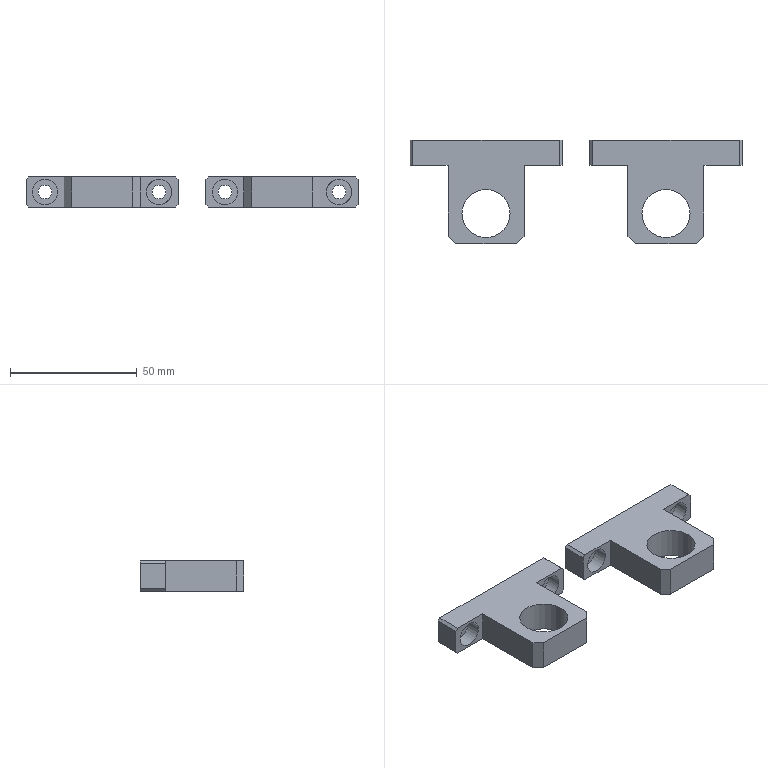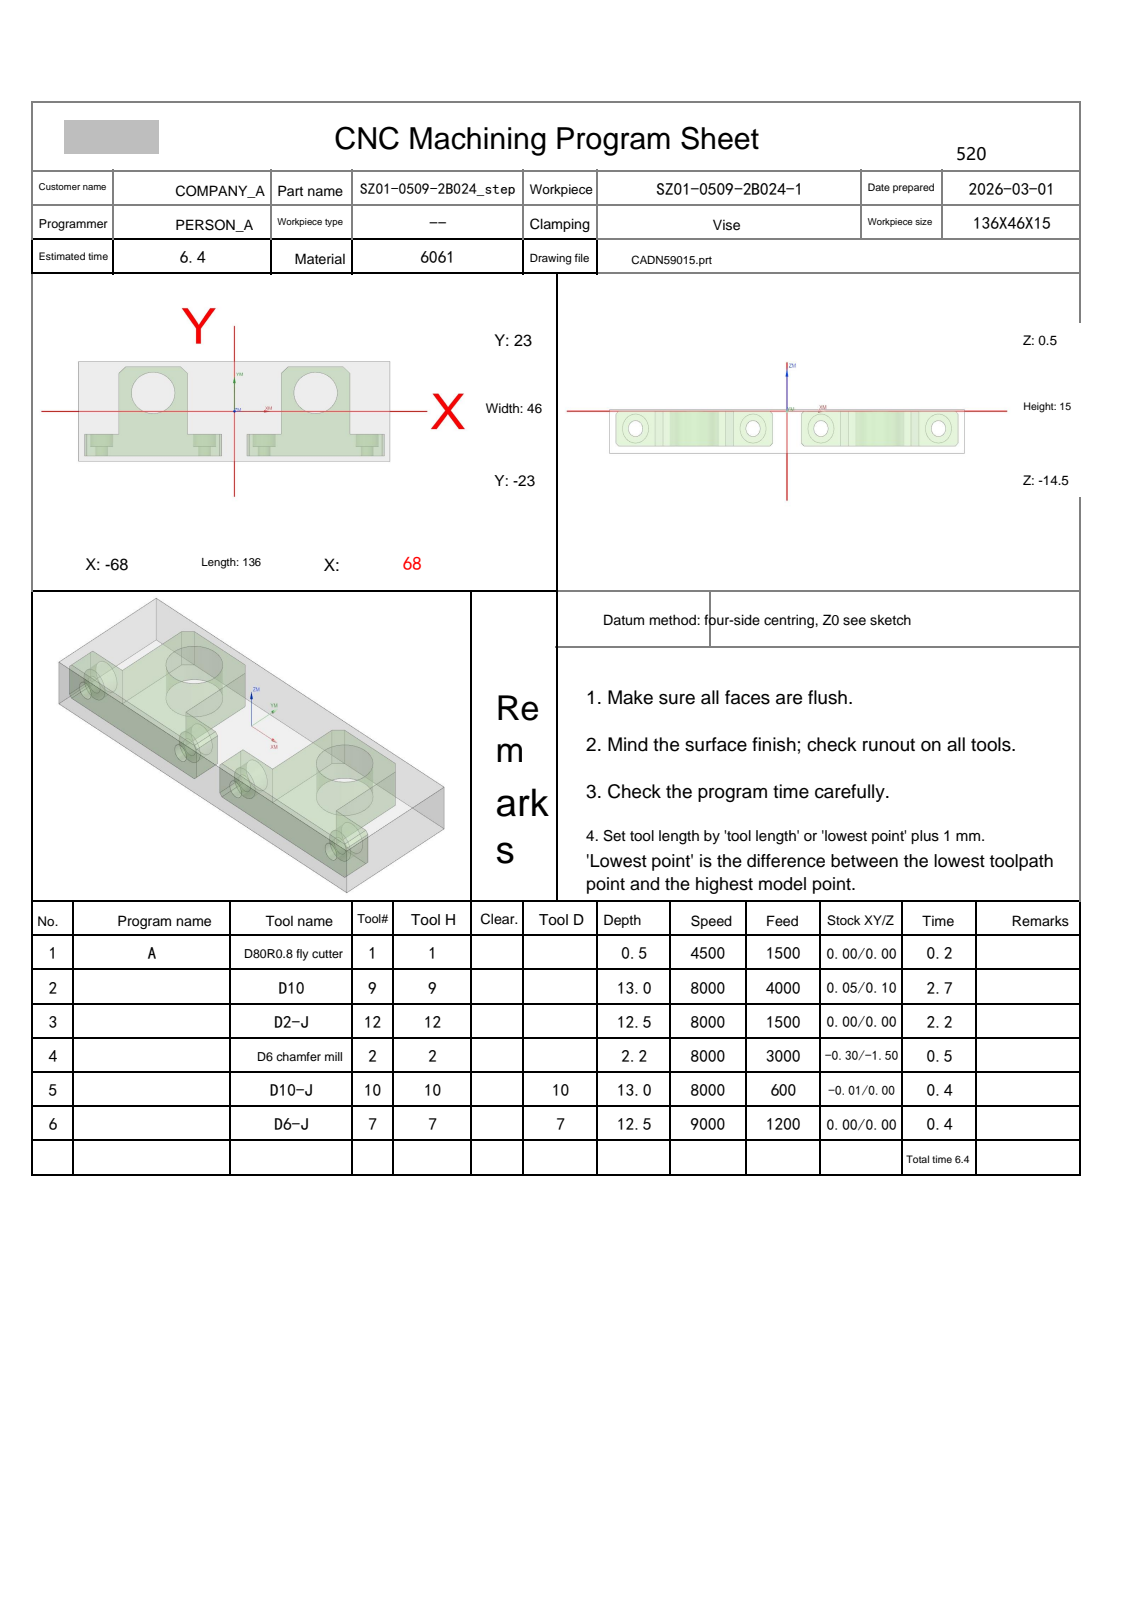NC program | NX | posted by the shop | part box 131 x 41 x 12 mm
Lines 2516 to 3597 of 8452:
N3 T12 M06
(D2-J  D=2. R=0. H=12 ce=0.00 di=0.00)
G00 G90 G54 X51.7 Y-5.35 M03 S8000
G43 H12 Z50.
M08
Z0.0
G01 X51.697 Y-5.351 Z-.03 F1500.
X51.69 Y-5.353 Z-.058
X51.679 Y-5.356 Z-.082
X51.665 Y-5.361 Z-.104
X51.648 Y-5.367 Z-.123
X51.63 Y-5.375 Z-.14
X51.61 Y-5.385 Z-.154
X51.59 Y-5.397 Z-.166
X51.57 Y-5.411 Z-.176
X51.552 Y-5.428 Z-.184
X51.535 Y-5.447 Z-.19
X51.521 Y-5.468 Z-.195
X51.51 Y-5.493 Z-.198
X51.503 Y-5.52 Z-.199
X51.5 Y-5.55 Z-.2
Y-9.5
X55.45
X55.464 Y-9.486 Z-.201
X55.453 Y-9.444 Z-.202
X55.419 Y-9.379 Z-.205
X55.364 Y-9.291 Z-.209
X55.099 Y-8.935 Z-.225
X54.845 Y-8.622 Z-.239
X54.646 Y-8.389 Z-.249
X54.409 Y-8.125 Z-.262
X54.132 Y-7.826 Z-.276
X53.822 Y-7.505 Z-.292
X53.495 Y-7.178 Z-.308
X53.174 Y-6.868 Z-.324
X52.875 Y-6.591 Z-.338
X52.611 Y-6.354 Z-.351
X52.378 Y-6.155 Z-.361
X52.065 Y-5.901 Z-.375
X51.709 Y-5.636 Z-.391
X51.621 Y-5.581 Z-.395
X51.556 Y-5.547 Z-.398
X51.514 Y-5.536 Z-.399
X51.5 Y-5.55 Z-.4
Y-9.5
X55.45
X55.464 Y-9.486 Z-.401
X55.453 Y-9.444 Z-.402
X55.419 Y-9.379 Z-.405
X55.364 Y-9.291 Z-.409
X55.099 Y-8.935 Z-.425
X54.845 Y-8.622 Z-.439
X54.646 Y-8.389 Z-.449
X54.409 Y-8.125 Z-.462
X54.132 Y-7.826 Z-.476
X53.822 Y-7.505 Z-.492
X53.495 Y-7.178 Z-.508
X53.174 Y-6.868 Z-.524
X52.875 Y-6.591 Z-.538
X52.611 Y-6.354 Z-.551
X52.378 Y-6.155 Z-.561
X52.065 Y-5.901 Z-.575
X51.709 Y-5.636 Z-.591
X51.621 Y-5.581 Z-.595
X51.556 Y-5.547 Z-.598
X51.514 Y-5.536 Z-.599
X51.5 Y-5.55 Z-.6
Y-9.5
X55.45
X55.464 Y-9.486 Z-.601
X55.453 Y-9.444 Z-.602
X55.419 Y-9.379 Z-.605
X55.364 Y-9.291 Z-.609
X55.099 Y-8.935 Z-.625
X54.845 Y-8.622 Z-.639
X54.646 Y-8.389 Z-.649
X54.409 Y-8.125 Z-.662
X54.132 Y-7.826 Z-.676
X53.822 Y-7.505 Z-.692
X53.495 Y-7.178 Z-.708
X53.174 Y-6.868 Z-.724
X52.875 Y-6.591 Z-.738
X52.611 Y-6.354 Z-.751
X52.378 Y-6.155 Z-.761
X52.065 Y-5.901 Z-.775
X51.709 Y-5.636 Z-.791
X51.621 Y-5.581 Z-.795
X51.556 Y-5.547 Z-.798
X51.514 Y-5.536 Z-.799
X51.5 Y-5.55 Z-.8
Y-9.5
X55.45
X55.464 Y-9.486 Z-.801
X55.453 Y-9.444 Z-.802
X55.419 Y-9.379 Z-.805
X55.364 Y-9.291 Z-.809
X55.099 Y-8.935 Z-.825
X54.845 Y-8.622 Z-.839
X54.646 Y-8.389 Z-.849
X54.409 Y-8.125 Z-.862
X54.132 Y-7.826 Z-.876
X53.822 Y-7.505 Z-.892
X53.495 Y-7.178 Z-.908
X53.174 Y-6.868 Z-.924
X52.875 Y-6.591 Z-.938
X52.611 Y-6.354 Z-.951
X52.378 Y-6.155 Z-.961
X52.065 Y-5.901 Z-.975
X51.709 Y-5.636 Z-.991
X51.621 Y-5.581 Z-.995
X51.556 Y-5.547 Z-.998
X51.514 Y-5.536 Z-.999
X51.5 Y-5.55 Z-1.
Y-9.5
X55.45
X55.464 Y-9.486 Z-1.001
X55.453 Y-9.444 Z-1.002
X55.419 Y-9.379 Z-1.005
X55.364 Y-9.291 Z-1.009
X55.099 Y-8.935 Z-1.025
X54.845 Y-8.622 Z-1.039
X54.646 Y-8.389 Z-1.049
X54.409 Y-8.125 Z-1.062
X54.132 Y-7.826 Z-1.076
X53.822 Y-7.505 Z-1.092
X53.495 Y-7.178 Z-1.108
X53.174 Y-6.868 Z-1.124
X52.875 Y-6.591 Z-1.138
X52.611 Y-6.354 Z-1.151
X52.378 Y-6.155 Z-1.161
X52.065 Y-5.901 Z-1.175
X51.709 Y-5.636 Z-1.191
X51.621 Y-5.581 Z-1.195
X51.556 Y-5.547 Z-1.198
X51.514 Y-5.536 Z-1.199
X51.5 Y-5.551 Z-1.2
Y-9.5
X55.45
X55.464 Y-9.486 Z-1.201
X55.453 Y-9.444 Z-1.202
X55.419 Y-9.379 Z-1.205
X55.364 Y-9.291 Z-1.209
X55.099 Y-8.935 Z-1.225
X54.845 Y-8.622 Z-1.239
X54.646 Y-8.389 Z-1.249
X54.409 Y-8.125 Z-1.262
X54.132 Y-7.826 Z-1.276
X53.822 Y-7.505 Z-1.292
X53.495 Y-7.178 Z-1.308
X53.174 Y-6.868 Z-1.324
X52.875 Y-6.591 Z-1.338
X52.611 Y-6.354 Z-1.351
X52.378 Y-6.155 Z-1.361
X52.065 Y-5.901 Z-1.375
X51.709 Y-5.636 Z-1.391
X51.621 Y-5.581 Z-1.395
X51.556 Y-5.547 Z-1.398
X51.514 Y-5.536 Z-1.399
X51.5 Y-5.551 Z-1.4
Y-9.5
X55.45
X55.464 Y-9.486 Z-1.401
X55.453 Y-9.444 Z-1.402
X55.419 Y-9.379 Z-1.405
X55.364 Y-9.291 Z-1.409
X55.099 Y-8.935 Z-1.425
X54.845 Y-8.622 Z-1.439
X54.646 Y-8.389 Z-1.449
X54.409 Y-8.125 Z-1.462
X54.132 Y-7.826 Z-1.476
X53.822 Y-7.505 Z-1.492
X53.495 Y-7.178 Z-1.508
X53.174 Y-6.868 Z-1.524
X52.875 Y-6.591 Z-1.538
X52.611 Y-6.354 Z-1.551
X52.378 Y-6.155 Z-1.561
X52.065 Y-5.901 Z-1.575
X51.709 Y-5.636 Z-1.591
X51.621 Y-5.581 Z-1.595
X51.556 Y-5.547 Z-1.598
X51.514 Y-5.536 Z-1.599
X51.5 Y-5.551 Z-1.6
Y-9.5
X55.45
X55.464 Y-9.486 Z-1.601
X55.453 Y-9.444 Z-1.602
X55.419 Y-9.379 Z-1.605
X55.364 Y-9.291 Z-1.609
X55.099 Y-8.935 Z-1.625
X54.845 Y-8.622 Z-1.639
X54.646 Y-8.389 Z-1.649
X54.409 Y-8.125 Z-1.662
X54.132 Y-7.826 Z-1.676
X53.822 Y-7.505 Z-1.692
X53.495 Y-7.178 Z-1.708
X53.174 Y-6.868 Z-1.724
X52.875 Y-6.591 Z-1.738
X52.611 Y-6.354 Z-1.751
X52.378 Y-6.155 Z-1.761
X52.065 Y-5.901 Z-1.775
X51.709 Y-5.636 Z-1.791
X51.621 Y-5.581 Z-1.795
X51.556 Y-5.547 Z-1.798
X51.514 Y-5.536 Z-1.799
X51.5 Y-5.551 Z-1.8
Y-9.5
X55.45
X55.464 Y-9.486 Z-1.801
X55.453 Y-9.444 Z-1.802
X55.419 Y-9.379 Z-1.805
X55.364 Y-9.291 Z-1.809
X55.099 Y-8.935 Z-1.825
X54.845 Y-8.622 Z-1.839
X54.646 Y-8.389 Z-1.849
X54.409 Y-8.125 Z-1.862
X54.132 Y-7.826 Z-1.876
X53.822 Y-7.505 Z-1.892
X53.495 Y-7.178 Z-1.908
X53.174 Y-6.868 Z-1.924
X52.875 Y-6.591 Z-1.938
X52.611 Y-6.354 Z-1.951
X52.378 Y-6.155 Z-1.961
X52.065 Y-5.901 Z-1.975
X51.709 Y-5.636 Z-1.991
X51.621 Y-5.581 Z-1.995
X51.556 Y-5.547 Z-1.998
X51.514 Y-5.536 Z-1.999
X51.5 Y-5.551 Z-2.
Y-9.5
X55.45
X55.464 Y-9.486 Z-2.001
X55.453 Y-9.444 Z-2.002
X55.419 Y-9.379 Z-2.005
X55.364 Y-9.291 Z-2.009
X55.099 Y-8.935 Z-2.025
X54.845 Y-8.622 Z-2.039
X54.646 Y-8.389 Z-2.049
X54.409 Y-8.125 Z-2.062
X54.132 Y-7.826 Z-2.076
X53.822 Y-7.505 Z-2.092
X53.495 Y-7.178 Z-2.108
X53.174 Y-6.868 Z-2.124
X52.875 Y-6.591 Z-2.138
X52.611 Y-6.354 Z-2.151
X52.378 Y-6.155 Z-2.161
X52.065 Y-5.901 Z-2.175
X51.709 Y-5.636 Z-2.191
X51.621 Y-5.581 Z-2.195
X51.556 Y-5.547 Z-2.198
X51.514 Y-5.536 Z-2.199
X51.5 Y-5.551 Z-2.2
Y-9.5
X55.45
X55.464 Y-9.486 Z-2.201
X55.453 Y-9.444 Z-2.202
X55.419 Y-9.379 Z-2.205
X55.364 Y-9.291 Z-2.209
X55.099 Y-8.935 Z-2.225
X54.845 Y-8.622 Z-2.239
X54.646 Y-8.389 Z-2.249
X54.409 Y-8.125 Z-2.262
X54.132 Y-7.826 Z-2.276
X53.822 Y-7.505 Z-2.292
X53.495 Y-7.178 Z-2.308
X53.174 Y-6.868 Z-2.324
X52.875 Y-6.591 Z-2.338
X52.611 Y-6.354 Z-2.351
X52.378 Y-6.155 Z-2.361
X52.065 Y-5.901 Z-2.375
X51.709 Y-5.636 Z-2.391
X51.621 Y-5.581 Z-2.395
X51.556 Y-5.547 Z-2.398
X51.514 Y-5.536 Z-2.399
X51.5 Y-5.551 Z-2.4
Y-9.5
X55.45
X55.464 Y-9.486 Z-2.401
X55.453 Y-9.444 Z-2.402
X55.419 Y-9.379 Z-2.405
X55.364 Y-9.291 Z-2.409
X55.099 Y-8.935 Z-2.425
X54.845 Y-8.622 Z-2.439
X54.646 Y-8.389 Z-2.449
X54.409 Y-8.125 Z-2.462
X54.132 Y-7.826 Z-2.476
X53.822 Y-7.505 Z-2.492
X53.495 Y-7.178 Z-2.508
X53.174 Y-6.868 Z-2.524
X52.875 Y-6.591 Z-2.538
X52.611 Y-6.354 Z-2.551
X52.378 Y-6.155 Z-2.561
X52.065 Y-5.901 Z-2.575
X51.709 Y-5.636 Z-2.591
X51.621 Y-5.581 Z-2.595
X51.556 Y-5.547 Z-2.598
X51.514 Y-5.536 Z-2.599
X51.5 Y-5.551 Z-2.6
Y-9.5
X55.45
X55.464 Y-9.486 Z-2.601
X55.453 Y-9.444 Z-2.602
X55.419 Y-9.379 Z-2.605
X55.364 Y-9.291 Z-2.609
X55.099 Y-8.935 Z-2.625
X54.845 Y-8.622 Z-2.639
X54.646 Y-8.389 Z-2.649
X54.409 Y-8.125 Z-2.662
X54.132 Y-7.826 Z-2.676
X53.822 Y-7.505 Z-2.692
X53.495 Y-7.178 Z-2.708
X53.174 Y-6.868 Z-2.724
X52.875 Y-6.591 Z-2.738
X52.611 Y-6.354 Z-2.751
X52.378 Y-6.155 Z-2.761
X52.065 Y-5.901 Z-2.775
X51.709 Y-5.636 Z-2.791
X51.621 Y-5.581 Z-2.795
X51.556 Y-5.547 Z-2.798
X51.514 Y-5.536 Z-2.799
X51.5 Y-5.551 Z-2.8
Y-9.5
X55.45
X55.464 Y-9.486 Z-2.801
X55.453 Y-9.444 Z-2.802
X55.419 Y-9.379 Z-2.805
X55.364 Y-9.291 Z-2.809
X55.099 Y-8.935 Z-2.825
X54.845 Y-8.622 Z-2.839
X54.646 Y-8.389 Z-2.849
X54.409 Y-8.125 Z-2.862
X54.132 Y-7.826 Z-2.876
X53.822 Y-7.505 Z-2.892
X53.495 Y-7.178 Z-2.908
X53.174 Y-6.868 Z-2.924
X52.875 Y-6.591 Z-2.938
X52.611 Y-6.354 Z-2.951
X52.378 Y-6.155 Z-2.961
X52.065 Y-5.901 Z-2.975
X51.709 Y-5.636 Z-2.991
X51.621 Y-5.581 Z-2.995
X51.556 Y-5.547 Z-2.998
X51.514 Y-5.536 Z-2.999
X51.5 Y-5.551 Z-3.
Y-9.5
X55.45
X55.464 Y-9.486 Z-3.001
X55.453 Y-9.444 Z-3.002
X55.419 Y-9.379 Z-3.005
X55.364 Y-9.291 Z-3.009
X55.099 Y-8.935 Z-3.025
X54.845 Y-8.622 Z-3.039
X54.646 Y-8.389 Z-3.049
X54.409 Y-8.125 Z-3.062
X54.132 Y-7.826 Z-3.076
X53.822 Y-7.505 Z-3.092
X53.495 Y-7.178 Z-3.108
X53.174 Y-6.868 Z-3.124
X52.875 Y-6.591 Z-3.138
X52.611 Y-6.354 Z-3.151
X52.378 Y-6.155 Z-3.161
X52.065 Y-5.901 Z-3.175
X51.709 Y-5.636 Z-3.191
X51.621 Y-5.581 Z-3.195
X51.556 Y-5.547 Z-3.198
X51.514 Y-5.536 Z-3.199
X51.5 Y-5.551 Z-3.2
Y-9.5
X55.45
X55.464 Y-9.486 Z-3.201
X55.453 Y-9.444 Z-3.202
X55.419 Y-9.379 Z-3.205
X55.364 Y-9.291 Z-3.209
X55.099 Y-8.935 Z-3.225
X54.845 Y-8.622 Z-3.239
X54.646 Y-8.389 Z-3.249
X54.409 Y-8.125 Z-3.262
X54.132 Y-7.826 Z-3.276
X53.822 Y-7.505 Z-3.292
X53.495 Y-7.178 Z-3.308
X53.174 Y-6.868 Z-3.324
X52.875 Y-6.591 Z-3.338
X52.611 Y-6.354 Z-3.351
X52.378 Y-6.155 Z-3.361
X52.065 Y-5.901 Z-3.375
X51.709 Y-5.636 Z-3.391
X51.621 Y-5.581 Z-3.395
X51.556 Y-5.547 Z-3.398
X51.514 Y-5.536 Z-3.399
X51.5 Y-5.551 Z-3.4
Y-9.5
X55.45
X55.464 Y-9.486 Z-3.401
X55.453 Y-9.444 Z-3.402
X55.419 Y-9.379 Z-3.405
X55.364 Y-9.291 Z-3.409
X55.099 Y-8.935 Z-3.425
X54.845 Y-8.622 Z-3.439
X54.646 Y-8.389 Z-3.449
X54.409 Y-8.125 Z-3.462
X54.132 Y-7.826 Z-3.476
X53.822 Y-7.505 Z-3.492
X53.495 Y-7.178 Z-3.508
X53.174 Y-6.868 Z-3.524
X52.875 Y-6.591 Z-3.538
X52.611 Y-6.354 Z-3.551
X52.378 Y-6.155 Z-3.561
X52.065 Y-5.901 Z-3.575
X51.709 Y-5.636 Z-3.591
X51.621 Y-5.581 Z-3.595
X51.556 Y-5.547 Z-3.598
X51.514 Y-5.536 Z-3.599
X51.5 Y-5.551 Z-3.6
Y-9.5
X55.45
X55.464 Y-9.486 Z-3.601
X55.453 Y-9.444 Z-3.602
X55.419 Y-9.379 Z-3.605
X55.364 Y-9.291 Z-3.609
X55.099 Y-8.935 Z-3.625
X54.845 Y-8.622 Z-3.639
X54.646 Y-8.389 Z-3.649
X54.409 Y-8.125 Z-3.662
X54.132 Y-7.826 Z-3.676
X53.822 Y-7.505 Z-3.692
X53.495 Y-7.178 Z-3.708
X53.174 Y-6.868 Z-3.724
X52.875 Y-6.591 Z-3.738
X52.611 Y-6.354 Z-3.751
X52.378 Y-6.155 Z-3.761
X52.065 Y-5.901 Z-3.775
X51.709 Y-5.636 Z-3.791
X51.621 Y-5.581 Z-3.795
X51.556 Y-5.547 Z-3.798
X51.514 Y-5.536 Z-3.799
X51.5 Y-5.551 Z-3.8
Y-9.5
X55.45
X55.464 Y-9.486 Z-3.801
X55.453 Y-9.444 Z-3.802
X55.419 Y-9.379 Z-3.805
X55.364 Y-9.291 Z-3.809
X55.099 Y-8.935 Z-3.825
X54.845 Y-8.622 Z-3.839
X54.646 Y-8.389 Z-3.849
X54.409 Y-8.125 Z-3.862
X54.132 Y-7.826 Z-3.876
X53.822 Y-7.505 Z-3.892
X53.495 Y-7.178 Z-3.908
X53.174 Y-6.868 Z-3.924
X52.875 Y-6.591 Z-3.938
X52.611 Y-6.354 Z-3.951
X52.378 Y-6.155 Z-3.961
X52.065 Y-5.901 Z-3.975
X51.709 Y-5.636 Z-3.991
X51.621 Y-5.581 Z-3.995
X51.556 Y-5.547 Z-3.998
X51.514 Y-5.536 Z-3.999
X51.5 Y-5.551 Z-4.
Y-9.5
X55.45
X55.464 Y-9.486 Z-4.001
X55.453 Y-9.444 Z-4.002
X55.419 Y-9.379 Z-4.005
X55.364 Y-9.291 Z-4.009
X55.099 Y-8.935 Z-4.025
X54.845 Y-8.622 Z-4.039
X54.646 Y-8.389 Z-4.049
X54.409 Y-8.125 Z-4.062
X54.132 Y-7.826 Z-4.076
X53.822 Y-7.505 Z-4.092
X53.495 Y-7.178 Z-4.108
X53.174 Y-6.868 Z-4.124
X52.875 Y-6.591 Z-4.138
X52.611 Y-6.354 Z-4.151
X52.378 Y-6.155 Z-4.161
X52.065 Y-5.901 Z-4.175
X51.709 Y-5.636 Z-4.191
X51.621 Y-5.581 Z-4.195
X51.556 Y-5.547 Z-4.198
X51.514 Y-5.536 Z-4.199
X51.5 Y-5.551 Z-4.2
Y-9.5
X55.45
X55.464 Y-9.486 Z-4.201
X55.453 Y-9.444 Z-4.202
X55.419 Y-9.379 Z-4.205
X55.364 Y-9.291 Z-4.209
X55.099 Y-8.935 Z-4.225
X54.845 Y-8.622 Z-4.239
X54.646 Y-8.389 Z-4.249
X54.409 Y-8.125 Z-4.262
X54.132 Y-7.826 Z-4.276
X53.822 Y-7.505 Z-4.292
X53.495 Y-7.178 Z-4.308
X53.174 Y-6.868 Z-4.324
X52.875 Y-6.591 Z-4.338
X52.611 Y-6.354 Z-4.351
X52.378 Y-6.155 Z-4.361
X52.065 Y-5.901 Z-4.375
X51.709 Y-5.636 Z-4.391
X51.621 Y-5.581 Z-4.395
X51.556 Y-5.547 Z-4.398
X51.514 Y-5.536 Z-4.399
X51.5 Y-5.551 Z-4.4
Y-9.5
X55.45
X55.464 Y-9.486 Z-4.401
X55.453 Y-9.444 Z-4.402
X55.419 Y-9.379 Z-4.405
X55.364 Y-9.291 Z-4.409
X55.099 Y-8.935 Z-4.425
X54.845 Y-8.622 Z-4.439
X54.646 Y-8.389 Z-4.449
X54.409 Y-8.125 Z-4.462
X54.132 Y-7.826 Z-4.476
X53.822 Y-7.505 Z-4.492
X53.495 Y-7.178 Z-4.508
X53.174 Y-6.868 Z-4.524
X52.875 Y-6.591 Z-4.538
X52.611 Y-6.354 Z-4.551
X52.378 Y-6.155 Z-4.561
X52.065 Y-5.901 Z-4.575
X51.709 Y-5.636 Z-4.591
X51.621 Y-5.581 Z-4.595
X51.556 Y-5.547 Z-4.598
X51.514 Y-5.536 Z-4.599
X51.5 Y-5.551 Z-4.6
Y-9.5
X55.45
X55.464 Y-9.486 Z-4.601
X55.453 Y-9.444 Z-4.602
X55.419 Y-9.379 Z-4.605
X55.364 Y-9.291 Z-4.609
X55.099 Y-8.935 Z-4.625
X54.845 Y-8.622 Z-4.639
X54.646 Y-8.389 Z-4.649
X54.409 Y-8.125 Z-4.662
X54.132 Y-7.826 Z-4.676
X53.822 Y-7.505 Z-4.692
X53.495 Y-7.178 Z-4.708
X53.174 Y-6.868 Z-4.724
X52.875 Y-6.591 Z-4.738
X52.611 Y-6.354 Z-4.751
X52.378 Y-6.155 Z-4.761
X52.065 Y-5.901 Z-4.775
X51.709 Y-5.636 Z-4.791
X51.621 Y-5.581 Z-4.795
X51.556 Y-5.547 Z-4.798
X51.514 Y-5.536 Z-4.799
X51.5 Y-5.551 Z-4.8
Y-9.5
X55.45
X55.464 Y-9.486 Z-4.801
X55.453 Y-9.444 Z-4.802
X55.419 Y-9.379 Z-4.805
X55.364 Y-9.291 Z-4.809
X55.099 Y-8.935 Z-4.825
X54.845 Y-8.622 Z-4.839
X54.646 Y-8.389 Z-4.849
X54.409 Y-8.125 Z-4.862
X54.132 Y-7.826 Z-4.876
X53.822 Y-7.505 Z-4.892
X53.495 Y-7.178 Z-4.908
X53.174 Y-6.868 Z-4.924
X52.875 Y-6.591 Z-4.938
X52.611 Y-6.354 Z-4.951
X52.378 Y-6.155 Z-4.961
X52.065 Y-5.901 Z-4.975
X51.709 Y-5.636 Z-4.991
X51.621 Y-5.581 Z-4.995
X51.556 Y-5.547 Z-4.998
X51.514 Y-5.536 Z-4.999
X51.5 Y-5.551 Z-5.
Y-9.5
X55.45
X55.464 Y-9.486 Z-5.001
X55.453 Y-9.444 Z-5.002
X55.419 Y-9.379 Z-5.005
X55.364 Y-9.291 Z-5.009
X55.099 Y-8.935 Z-5.025
X54.845 Y-8.622 Z-5.039
X54.646 Y-8.389 Z-5.049
X54.409 Y-8.125 Z-5.062
X54.132 Y-7.826 Z-5.076
X53.822 Y-7.505 Z-5.092
X53.495 Y-7.178 Z-5.108
X53.174 Y-6.868 Z-5.124
X52.875 Y-6.591 Z-5.138
X52.611 Y-6.354 Z-5.151
X52.378 Y-6.155 Z-5.161
X52.065 Y-5.901 Z-5.175
X51.709 Y-5.636 Z-5.191
X51.621 Y-5.581 Z-5.195
X51.556 Y-5.547 Z-5.198
X51.514 Y-5.536 Z-5.199
X51.5 Y-5.551 Z-5.2
Y-9.5
X55.45
X55.464 Y-9.486 Z-5.201
X55.453 Y-9.444 Z-5.202
X55.419 Y-9.379 Z-5.205
X55.364 Y-9.291 Z-5.209
X55.099 Y-8.935 Z-5.225
X54.845 Y-8.622 Z-5.239
X54.646 Y-8.389 Z-5.249
X54.409 Y-8.125 Z-5.262
X54.132 Y-7.826 Z-5.276
X53.822 Y-7.505 Z-5.292
X53.495 Y-7.178 Z-5.308
X53.174 Y-6.868 Z-5.324
X52.875 Y-6.591 Z-5.338
X52.611 Y-6.354 Z-5.351
X52.378 Y-6.155 Z-5.361
X52.065 Y-5.901 Z-5.375
X51.709 Y-5.636 Z-5.391
X51.621 Y-5.581 Z-5.395
X51.556 Y-5.547 Z-5.398
X51.514 Y-5.536 Z-5.399
X51.5 Y-5.551 Z-5.4
Y-9.5
X55.45
X55.464 Y-9.486 Z-5.401
X55.453 Y-9.444 Z-5.402
X55.419 Y-9.379 Z-5.405
X55.364 Y-9.291 Z-5.409
X55.099 Y-8.935 Z-5.425
X54.845 Y-8.622 Z-5.439
X54.646 Y-8.389 Z-5.449
X54.409 Y-8.125 Z-5.462
X54.132 Y-7.826 Z-5.476
X53.822 Y-7.505 Z-5.492
X53.495 Y-7.178 Z-5.508
X53.174 Y-6.868 Z-5.524
X52.875 Y-6.591 Z-5.538
X52.611 Y-6.354 Z-5.551
X52.378 Y-6.155 Z-5.561
X52.065 Y-5.901 Z-5.575
X51.709 Y-5.636 Z-5.591
X51.621 Y-5.581 Z-5.595
X51.556 Y-5.547 Z-5.598
X51.514 Y-5.536 Z-5.599
X51.5 Y-5.551 Z-5.6
Y-9.5
X55.45
X55.464 Y-9.486 Z-5.601
X55.453 Y-9.444 Z-5.602
X55.419 Y-9.379 Z-5.605
X55.364 Y-9.291 Z-5.609
X55.099 Y-8.935 Z-5.625
X54.845 Y-8.622 Z-5.639
X54.646 Y-8.389 Z-5.649
X54.409 Y-8.125 Z-5.662
X54.132 Y-7.826 Z-5.676
X53.822 Y-7.505 Z-5.692
X53.495 Y-7.178 Z-5.708
X53.174 Y-6.868 Z-5.724
X52.875 Y-6.591 Z-5.738
X52.611 Y-6.354 Z-5.751
X52.378 Y-6.155 Z-5.761
X52.065 Y-5.901 Z-5.775
X51.709 Y-5.636 Z-5.791
X51.621 Y-5.581 Z-5.795
X51.556 Y-5.547 Z-5.798
X51.514 Y-5.536 Z-5.799
X51.5 Y-5.551 Z-5.8
Y-9.5
X55.45
X55.464 Y-9.486 Z-5.801
X55.453 Y-9.444 Z-5.802
X55.419 Y-9.379 Z-5.805
X55.364 Y-9.291 Z-5.809
X55.099 Y-8.935 Z-5.825
X54.845 Y-8.622 Z-5.839
X54.646 Y-8.389 Z-5.849
X54.409 Y-8.125 Z-5.862
X54.132 Y-7.826 Z-5.876
X53.822 Y-7.505 Z-5.892
X53.495 Y-7.178 Z-5.908
X53.174 Y-6.868 Z-5.924
X52.875 Y-6.591 Z-5.938
X52.611 Y-6.354 Z-5.951
X52.378 Y-6.155 Z-5.961
X52.065 Y-5.901 Z-5.975
X51.709 Y-5.636 Z-5.991
X51.621 Y-5.581 Z-5.995
X51.556 Y-5.547 Z-5.998
X51.514 Y-5.536 Z-5.999
X51.5 Y-5.551 Z-6.
Y-9.5
X55.45
X55.464 Y-9.486 Z-6.001
X55.453 Y-9.444 Z-6.002
X55.419 Y-9.379 Z-6.005
X55.364 Y-9.291 Z-6.009
X55.099 Y-8.935 Z-6.025
X54.845 Y-8.622 Z-6.039
X54.646 Y-8.389 Z-6.049
X54.409 Y-8.125 Z-6.062
X54.132 Y-7.826 Z-6.076
X53.822 Y-7.505 Z-6.092
X53.495 Y-7.178 Z-6.108
X53.174 Y-6.868 Z-6.124
X52.875 Y-6.591 Z-6.138
X52.611 Y-6.354 Z-6.151
X52.378 Y-6.155 Z-6.161
X52.065 Y-5.901 Z-6.175
X51.709 Y-5.636 Z-6.191
X51.621 Y-5.581 Z-6.195
X51.556 Y-5.547 Z-6.198
X51.514 Y-5.536 Z-6.199
X51.5 Y-5.551 Z-6.2
Y-9.5
X55.45
X55.464 Y-9.486 Z-6.201
X55.453 Y-9.444 Z-6.202
X55.419 Y-9.379 Z-6.205
X55.364 Y-9.291 Z-6.209
X55.099 Y-8.935 Z-6.225
X54.845 Y-8.622 Z-6.239
X54.646 Y-8.389 Z-6.249
X54.409 Y-8.125 Z-6.262
X54.132 Y-7.826 Z-6.276
X53.822 Y-7.505 Z-6.292
X53.495 Y-7.178 Z-6.308
X53.174 Y-6.868 Z-6.324
X52.875 Y-6.591 Z-6.338
X52.611 Y-6.354 Z-6.351
X52.378 Y-6.155 Z-6.361
X52.065 Y-5.901 Z-6.375
X51.709 Y-5.636 Z-6.391
X51.621 Y-5.581 Z-6.395
X51.556 Y-5.547 Z-6.398
X51.514 Y-5.536 Z-6.399
X51.5 Y-5.551 Z-6.4
Y-9.5
X55.45
X55.464 Y-9.486 Z-6.401
X55.453 Y-9.444 Z-6.402
X55.419 Y-9.379 Z-6.405
X55.364 Y-9.291 Z-6.409
X55.099 Y-8.935 Z-6.425
X54.845 Y-8.622 Z-6.439
X54.646 Y-8.389 Z-6.449
X54.409 Y-8.125 Z-6.462
X54.132 Y-7.826 Z-6.476
X53.822 Y-7.505 Z-6.492
X53.495 Y-7.178 Z-6.508
X53.174 Y-6.868 Z-6.524
X52.875 Y-6.591 Z-6.538
X52.611 Y-6.354 Z-6.551
X52.378 Y-6.155 Z-6.561
X52.065 Y-5.901 Z-6.575
X51.709 Y-5.636 Z-6.591
X51.621 Y-5.581 Z-6.595
X51.556 Y-5.547 Z-6.598
X51.514 Y-5.536 Z-6.599
X51.5 Y-5.551 Z-6.6
Y-9.5
X55.45
X55.464 Y-9.486 Z-6.601
X55.453 Y-9.444 Z-6.602
X55.419 Y-9.379 Z-6.605
X55.364 Y-9.291 Z-6.609
X55.099 Y-8.935 Z-6.625
X54.845 Y-8.622 Z-6.639
X54.646 Y-8.389 Z-6.649
X54.409 Y-8.125 Z-6.662
X54.132 Y-7.826 Z-6.676
X53.822 Y-7.505 Z-6.692
X53.495 Y-7.178 Z-6.708
X53.174 Y-6.868 Z-6.724
X52.875 Y-6.591 Z-6.738
X52.611 Y-6.354 Z-6.751
X52.378 Y-6.155 Z-6.761
X52.065 Y-5.901 Z-6.775
X51.709 Y-5.636 Z-6.791
X51.621 Y-5.581 Z-6.795
X51.556 Y-5.547 Z-6.798
X51.514 Y-5.536 Z-6.799
X51.5 Y-5.551 Z-6.8
Y-9.5
X55.45
X55.464 Y-9.486 Z-6.801
X55.453 Y-9.444 Z-6.802
X55.419 Y-9.379 Z-6.805
X55.364 Y-9.291 Z-6.809
X55.099 Y-8.935 Z-6.825
X54.845 Y-8.622 Z-6.839
X54.646 Y-8.389 Z-6.849
X54.409 Y-8.125 Z-6.862
X54.132 Y-7.826 Z-6.876
X53.822 Y-7.505 Z-6.892
X53.495 Y-7.178 Z-6.908
X53.174 Y-6.868 Z-6.924
X52.875 Y-6.591 Z-6.938
X52.611 Y-6.354 Z-6.951
X52.378 Y-6.155 Z-6.961
X52.065 Y-5.901 Z-6.975
X51.709 Y-5.636 Z-6.991
X51.621 Y-5.581 Z-6.995
X51.556 Y-5.547 Z-6.998
X51.514 Y-5.536 Z-6.999
X51.5 Y-5.551 Z-7.
Y-9.5
X55.45
X55.464 Y-9.486 Z-7.001
X55.453 Y-9.444 Z-7.002
X55.419 Y-9.379 Z-7.005
X55.364 Y-9.291 Z-7.009
X55.099 Y-8.935 Z-7.025
X54.845 Y-8.622 Z-7.039
X54.646 Y-8.389 Z-7.049
X54.409 Y-8.125 Z-7.062
X54.132 Y-7.826 Z-7.076
X53.822 Y-7.505 Z-7.092
X53.495 Y-7.178 Z-7.108
X53.174 Y-6.868 Z-7.124
X52.875 Y-6.591 Z-7.138
X52.611 Y-6.354 Z-7.151
X52.378 Y-6.155 Z-7.161
X52.065 Y-5.901 Z-7.175
X51.709 Y-5.636 Z-7.191
X51.621 Y-5.581 Z-7.195
X51.556 Y-5.547 Z-7.198
X51.514 Y-5.536 Z-7.199
X51.5 Y-5.551 Z-7.2
Y-9.5
X55.45
X55.464 Y-9.486 Z-7.201
X55.453 Y-9.444 Z-7.202
X55.419 Y-9.379 Z-7.205
X55.364 Y-9.291 Z-7.209
X55.099 Y-8.935 Z-7.225
X54.845 Y-8.622 Z-7.239
X54.646 Y-8.389 Z-7.249
X54.409 Y-8.125 Z-7.262
X54.132 Y-7.826 Z-7.276
X53.822 Y-7.505 Z-7.292
X53.495 Y-7.178 Z-7.308
X53.174 Y-6.868 Z-7.324
X52.875 Y-6.591 Z-7.338
X52.611 Y-6.354 Z-7.351
X52.378 Y-6.155 Z-7.361
X52.065 Y-5.901 Z-7.375
X51.709 Y-5.636 Z-7.391
X51.621 Y-5.581 Z-7.395
X51.556 Y-5.547 Z-7.398
X51.514 Y-5.536 Z-7.399
X51.5 Y-5.551 Z-7.4
Y-9.5
X55.45
X55.464 Y-9.486 Z-7.401
X55.453 Y-9.444 Z-7.402
X55.419 Y-9.379 Z-7.405
X55.364 Y-9.291 Z-7.409
X55.099 Y-8.935 Z-7.425
X54.845 Y-8.622 Z-7.439
X54.646 Y-8.389 Z-7.449
X54.409 Y-8.125 Z-7.462
X54.132 Y-7.826 Z-7.476
X53.822 Y-7.505 Z-7.492
X53.495 Y-7.178 Z-7.508
X53.174 Y-6.868 Z-7.524
X52.875 Y-6.591 Z-7.538
X52.611 Y-6.354 Z-7.551
X52.378 Y-6.155 Z-7.561
X52.065 Y-5.901 Z-7.575
X51.709 Y-5.636 Z-7.591
X51.621 Y-5.581 Z-7.595
X51.556 Y-5.547 Z-7.598
X51.514 Y-5.536 Z-7.599
X51.5 Y-5.551 Z-7.6
Y-9.5
X55.45
X55.464 Y-9.486 Z-7.601
X55.453 Y-9.444 Z-7.602
X55.419 Y-9.379 Z-7.605
X55.364 Y-9.291 Z-7.609
X55.099 Y-8.935 Z-7.625
X54.845 Y-8.622 Z-7.639
X54.646 Y-8.389 Z-7.649
X54.409 Y-8.125 Z-7.662
X54.132 Y-7.826 Z-7.676
X53.822 Y-7.505 Z-7.692
X53.495 Y-7.178 Z-7.708
X53.174 Y-6.868 Z-7.724
X52.875 Y-6.591 Z-7.738
X52.611 Y-6.354 Z-7.751
X52.378 Y-6.155 Z-7.761
X52.065 Y-5.901 Z-7.775
X51.709 Y-5.636 Z-7.791
X51.621 Y-5.581 Z-7.795
X51.556 Y-5.547 Z-7.798
X51.514 Y-5.536 Z-7.799
X51.5 Y-5.551 Z-7.8
Y-9.5
X55.45
X55.464 Y-9.486 Z-7.801
X55.453 Y-9.444 Z-7.802
X55.419 Y-9.379 Z-7.805
X55.364 Y-9.291 Z-7.809
X55.099 Y-8.935 Z-7.825
X54.845 Y-8.622 Z-7.839
X54.646 Y-8.389 Z-7.849
X54.409 Y-8.125 Z-7.862
X54.132 Y-7.826 Z-7.876
X53.822 Y-7.505 Z-7.892
X53.495 Y-7.178 Z-7.908
X53.174 Y-6.868 Z-7.924
X52.875 Y-6.591 Z-7.938
X52.611 Y-6.354 Z-7.951
X52.378 Y-6.155 Z-7.961
X52.065 Y-5.901 Z-7.975
X51.709 Y-5.636 Z-7.991
X51.621 Y-5.581 Z-7.995
X51.556 Y-5.547 Z-7.998
X51.514 Y-5.536 Z-7.999
X51.5 Y-5.551 Z-8.
Y-9.5
X55.45
X55.464 Y-9.486 Z-8.001
X55.453 Y-9.444 Z-8.002
X55.419 Y-9.379 Z-8.005
X55.364 Y-9.291 Z-8.009
X55.099 Y-8.935 Z-8.025
X54.845 Y-8.622 Z-8.039
X54.646 Y-8.389 Z-8.049
X54.409 Y-8.125 Z-8.062
X54.132 Y-7.826 Z-8.076
X53.822 Y-7.505 Z-8.092
X53.495 Y-7.178 Z-8.108
X53.174 Y-6.868 Z-8.124
X52.875 Y-6.591 Z-8.138
X52.611 Y-6.354 Z-8.151
X52.378 Y-6.155 Z-8.161
X52.065 Y-5.901 Z-8.175
X51.709 Y-5.636 Z-8.191
X51.621 Y-5.581 Z-8.195
X51.556 Y-5.547 Z-8.198
X51.514 Y-5.536 Z-8.199
X51.5 Y-5.551 Z-8.2
Y-9.5
X55.45
X55.464 Y-9.486 Z-8.201
X55.453 Y-9.444 Z-8.202
X55.419 Y-9.379 Z-8.205
X55.364 Y-9.291 Z-8.209
X55.099 Y-8.935 Z-8.225
X54.845 Y-8.622 Z-8.239
X54.646 Y-8.389 Z-8.249
X54.409 Y-8.125 Z-8.262
X54.132 Y-7.826 Z-8.276
X53.822 Y-7.505 Z-8.292
X53.495 Y-7.178 Z-8.308
X53.174 Y-6.868 Z-8.324
X52.875 Y-6.591 Z-8.338
X52.611 Y-6.354 Z-8.351
X52.378 Y-6.155 Z-8.361
X52.065 Y-5.901 Z-8.375
X51.709 Y-5.636 Z-8.391
X51.621 Y-5.581 Z-8.395
X51.556 Y-5.547 Z-8.398
X51.514 Y-5.536 Z-8.399
X51.5 Y-5.551 Z-8.4
Y-9.5
X55.45
X55.464 Y-9.486 Z-8.401
X55.453 Y-9.444 Z-8.402
X55.419 Y-9.379 Z-8.405
X55.364 Y-9.291 Z-8.409
X55.099 Y-8.935 Z-8.425
X54.845 Y-8.622 Z-8.439
X54.646 Y-8.389 Z-8.449
X54.409 Y-8.125 Z-8.462
X54.132 Y-7.826 Z-8.476
X53.822 Y-7.505 Z-8.492
X53.495 Y-7.178 Z-8.508
X53.174 Y-6.868 Z-8.524
X52.875 Y-6.591 Z-8.538
X52.611 Y-6.354 Z-8.551
X52.378 Y-6.155 Z-8.561
X52.065 Y-5.901 Z-8.575
X51.709 Y-5.636 Z-8.591
X51.621 Y-5.581 Z-8.595
X51.556 Y-5.547 Z-8.598
X51.514 Y-5.536 Z-8.599
X51.5 Y-5.551 Z-8.6
Y-9.5
X55.45
X55.464 Y-9.486 Z-8.601
X55.453 Y-9.444 Z-8.602
X55.419 Y-9.379 Z-8.605
X55.364 Y-9.291 Z-8.609
X55.099 Y-8.935 Z-8.625
X54.845 Y-8.622 Z-8.639
X54.646 Y-8.389 Z-8.649
X54.409 Y-8.125 Z-8.662
X54.132 Y-7.826 Z-8.676
X53.822 Y-7.505 Z-8.692
X53.495 Y-7.178 Z-8.708
X53.174 Y-6.868 Z-8.724
X52.875 Y-6.591 Z-8.738
X52.611 Y-6.354 Z-8.751
X52.378 Y-6.155 Z-8.761
X52.065 Y-5.901 Z-8.775
X51.709 Y-5.636 Z-8.791
X51.621 Y-5.581 Z-8.795
X51.556 Y-5.547 Z-8.798
X51.514 Y-5.536 Z-8.799
X51.5 Y-5.551 Z-8.8
Y-9.5
X55.45
X55.464 Y-9.486 Z-8.801
X55.453 Y-9.444 Z-8.802
X55.419 Y-9.379 Z-8.805
X55.364 Y-9.291 Z-8.809
X55.099 Y-8.935 Z-8.825
X54.845 Y-8.622 Z-8.839
X54.646 Y-8.389 Z-8.849
X54.409 Y-8.125 Z-8.862
X54.132 Y-7.826 Z-8.876
X53.822 Y-7.505 Z-8.892
X53.495 Y-7.178 Z-8.908
X53.174 Y-6.868 Z-8.924
X52.875 Y-6.591 Z-8.938
X52.611 Y-6.354 Z-8.951
X52.378 Y-6.155 Z-8.961
X52.065 Y-5.901 Z-8.975
X51.709 Y-5.636 Z-8.991
X51.621 Y-5.581 Z-8.995
X51.556 Y-5.547 Z-8.998
X51.514 Y-5.536 Z-8.999
X51.5 Y-5.551 Z-9.
Y-9.5
X55.45
X55.464 Y-9.486 Z-9.001
X55.453 Y-9.444 Z-9.002
X55.419 Y-9.379 Z-9.005
X55.364 Y-9.291 Z-9.009
X55.099 Y-8.935 Z-9.025
X54.845 Y-8.622 Z-9.039
X54.646 Y-8.389 Z-9.049
X54.409 Y-8.125 Z-9.062
X54.132 Y-7.826 Z-9.076
X53.822 Y-7.505 Z-9.092
X53.495 Y-7.178 Z-9.108
X53.174 Y-6.868 Z-9.124
X52.875 Y-6.591 Z-9.138
X52.611 Y-6.354 Z-9.151
X52.378 Y-6.155 Z-9.161
X52.065 Y-5.901 Z-9.175
X51.709 Y-5.636 Z-9.191
X51.621 Y-5.581 Z-9.195
X51.556 Y-5.547 Z-9.198
X51.514 Y-5.536 Z-9.199
X51.5 Y-5.551 Z-9.2
Y-9.5
X55.45
X55.464 Y-9.486 Z-9.201
X55.453 Y-9.444 Z-9.202
X55.419 Y-9.379 Z-9.205
X55.364 Y-9.291 Z-9.209
X55.099 Y-8.935 Z-9.225
X54.845 Y-8.622 Z-9.239
X54.646 Y-8.389 Z-9.249
X54.409 Y-8.125 Z-9.262
X54.132 Y-7.826 Z-9.276
X53.822 Y-7.505 Z-9.292
X53.495 Y-7.178 Z-9.308
X53.174 Y-6.868 Z-9.324
X52.875 Y-6.591 Z-9.338
X52.611 Y-6.354 Z-9.351
X52.378 Y-6.155 Z-9.361
X52.065 Y-5.901 Z-9.375
X51.709 Y-5.636 Z-9.391
X51.621 Y-5.581 Z-9.395
X51.556 Y-5.547 Z-9.398
X51.514 Y-5.536 Z-9.399
X51.5 Y-5.551 Z-9.4
Y-9.5
X55.45
X55.464 Y-9.486 Z-9.401